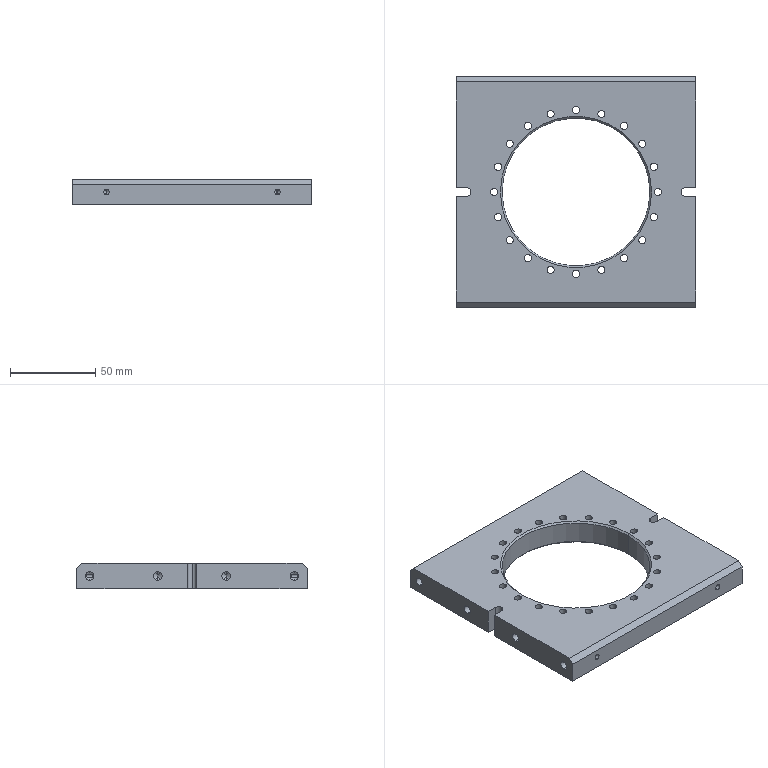Part | SolidWorks | features HoleWzd 3, Chamfer 2, MirrorPattern 2, CirPattern 1, Extrusion 1, ICE 1 | 1 solid | 111 faces | box 140 x 135 x 15 mm | volume 184976 mm3 | cylinder 69 | cone 28 | plane 14 | commonest cylinder face diameters 4.2 x40 5 x19 3.3 x8 86.5 x2